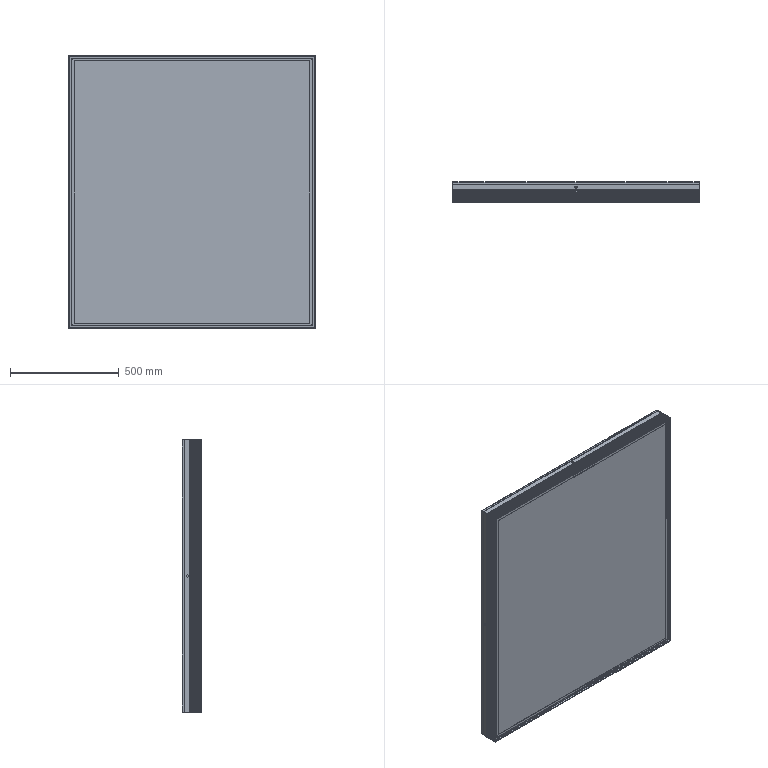Part | SolidWorks | 50 solids | 3317 faces | volume 187293162 mm3 | plane 2111 | cylinder 1094 | spline 112 | commonest cylinder face diameters 7 x360 0.4 x165 11 x134 2.4 x113 0.6 x80 4.2 x80